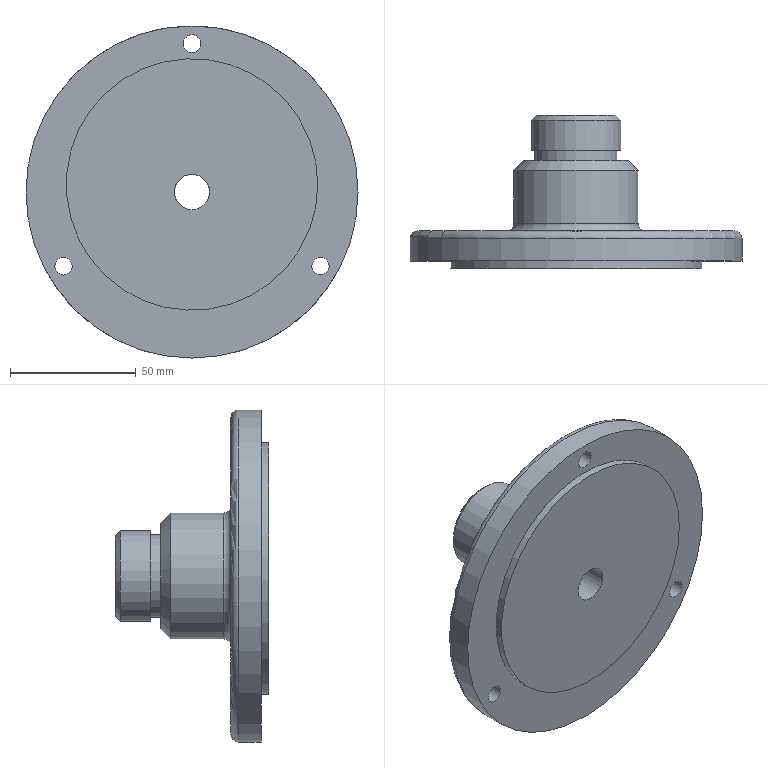Part | NX | features DATUM_CSYS 7, SKETCH 6, CBORE_HOLE 3, EXTRACT_FACE 3, EXTRUDE 3, HOLE PACKAGE 3, CHAMFER 2, Instance Feature 2, BLEND 1, Pattern Feature 1, SWP104 1 | 1 solid | 27 faces | box 132 x 61 x 132 mm | volume 237837 mm3 | cylinder 13 | plane 9 | cone 3 | torus 2 | commonest cylinder face diameters 7 x3 11 x3 14 x1 25 x1 33 x1 36 x1
STEP:
#1=CARTESIAN_POINT('',(50.,0.,3.));
#2=VERTEX_POINT('',#1);
#3=CARTESIAN_POINT('',(0.,0.,3.));
#4=DIRECTION('',(0.,-1.,0.));
#5=DIRECTION('',(1.,0.,0.));
#6=AXIS2_PLACEMENT_3D('',#3,#4,#5);
#7=CIRCLE('',#6,50.);
#8=EDGE_CURVE('',#2,#2,#7,.T.);
#9=ORIENTED_EDGE('',*,*,#8,.T.);
#10=EDGE_LOOP('',(#9));
#11=FACE_BOUND('',#10,.T.);
#12=CARTESIAN_POINT('',(50.,-3.,3.));
#13=VERTEX_POINT('',#12);
#14=CARTESIAN_POINT('',(0.,-3.,3.));
#15=DIRECTION('',(0.,-1.,0.));
#16=DIRECTION('',(1.,0.,0.));
#17=AXIS2_PLACEMENT_3D('',#14,#15,#16);
#18=CIRCLE('',#17,50.);
#19=EDGE_CURVE('',#13,#13,#18,.T.);
#20=ORIENTED_EDGE('',*,*,#19,.F.);
#21=EDGE_LOOP('',(#20));
#22=FACE_BOUND('',#21,.T.);
#23=CARTESIAN_POINT('',(0.,-3.,3.));
#24=DIRECTION('',(0.,1.,0.));
#25=DIRECTION('',(0.,0.,1.));
#26=AXIS2_PLACEMENT_3D('',#23,#24,#25);
#27=CYLINDRICAL_SURFACE('',#26,50.);
#28=ADVANCED_FACE('',(#11,#22),#27,.T.);
#29=CARTESIAN_POINT('',(7.,-3.,0.));
#30=VERTEX_POINT('',#29);
#31=CARTESIAN_POINT('',(0.,-3.,0.));
#32=DIRECTION('',(0.,-1.,0.));
#33=DIRECTION('',(1.,0.,0.));
#34=AXIS2_PLACEMENT_3D('',#31,#32,#33);
#35=CIRCLE('',#34,7.);
#36=EDGE_CURVE('',#30,#30,#35,.T.);
#37=ORIENTED_EDGE('',*,*,#36,.F.);
#38=EDGE_LOOP('',(#37));
#39=FACE_BOUND('',#38,.T.);
#40=ORIENTED_EDGE('',*,*,#19,.T.);
#41=EDGE_LOOP('',(#40));
#42=FACE_BOUND('',#41,.T.);
#43=CARTESIAN_POINT('',(0.,-3.,3.));
#44=DIRECTION('',(0.,-1.,0.));
#45=DIRECTION('',(0.,0.,-1.));
#46=AXIS2_PLACEMENT_3D('',#43,#44,#45);
#47=PLANE('',#46);
#48=ADVANCED_FACE('',(#39,#42),#47,.T.);
#49=CARTESIAN_POINT('',(0.,9.,-66.));
#50=VERTEX_POINT('',#49);
#51=CARTESIAN_POINT('',(0.,9.,0.));
#52=DIRECTION('',(0.,-1.,0.));
#53=DIRECTION('',(0.,0.,-1.));
#54=AXIS2_PLACEMENT_3D('',#51,#52,#53);
#55=CIRCLE('',#54,66.);
#56=EDGE_CURVE('',#50,#50,#55,.T.);
#57=ORIENTED_EDGE('',*,*,#56,.T.);
#58=EDGE_LOOP('',(#57));
#59=FACE_BOUND('',#58,.T.);
#60=CARTESIAN_POINT('',(66.,0.,0.));
#61=VERTEX_POINT('',#60);
#62=CARTESIAN_POINT('',(0.,0.,0.));
#63=DIRECTION('',(0.,-1.,0.));
#64=DIRECTION('',(1.,0.,0.));
#65=AXIS2_PLACEMENT_3D('',#62,#63,#64);
#66=CIRCLE('',#65,66.);
#67=EDGE_CURVE('',#61,#61,#66,.T.);
#68=ORIENTED_EDGE('',*,*,#67,.F.);
#69=EDGE_LOOP('',(#68));
#70=FACE_BOUND('',#69,.T.);
#71=CARTESIAN_POINT('',(0.,12.,0.));
#72=DIRECTION('',(0.,-1.,0.));
#73=DIRECTION('',(0.,0.,-1.));
#74=AXIS2_PLACEMENT_3D('',#71,#72,#73);
#75=CYLINDRICAL_SURFACE('',#74,66.);
#76=ADVANCED_FACE('',(#59,#70),#75,.T.);
#77=CARTESIAN_POINT('',(-51.095,0.,-33.));
#78=VERTEX_POINT('',#77);
#79=CARTESIAN_POINT('',(-51.095,0.,-29.5));
#80=DIRECTION('',(0.,-1.,0.));
#81=DIRECTION('',(0.,0.,-1.));
#82=AXIS2_PLACEMENT_3D('',#79,#80,#81);
#83=CIRCLE('',#82,3.5);
#84=EDGE_CURVE('',#78,#78,#83,.T.);
#85=ORIENTED_EDGE('',*,*,#84,.F.);
#86=EDGE_LOOP('',(#85));
#87=FACE_BOUND('',#86,.T.);
#88=CARTESIAN_POINT('',(51.095,0.,-33.));
#89=VERTEX_POINT('',#88);
#90=CARTESIAN_POINT('',(51.095,0.,-29.5));
#91=DIRECTION('',(0.,-1.,0.));
#92=DIRECTION('',(0.,0.,-1.));
#93=AXIS2_PLACEMENT_3D('',#90,#91,#92);
#94=CIRCLE('',#93,3.5);
#95=EDGE_CURVE('',#89,#89,#94,.T.);
#96=ORIENTED_EDGE('',*,*,#95,.F.);
#97=EDGE_LOOP('',(#96));
#98=FACE_BOUND('',#97,.T.);
#99=CARTESIAN_POINT('',(0.,0.,55.5));
#100=VERTEX_POINT('',#99);
#101=CARTESIAN_POINT('',(0.,0.,59.));
#102=DIRECTION('',(0.,-1.,0.));
#103=DIRECTION('',(0.,0.,-1.));
#104=AXIS2_PLACEMENT_3D('',#101,#102,#103);
#105=CIRCLE('',#104,3.5);
#106=EDGE_CURVE('',#100,#100,#105,.T.);
#107=ORIENTED_EDGE('',*,*,#106,.F.);
#108=EDGE_LOOP('',(#107));
#109=FACE_BOUND('',#108,.T.);
#110=ORIENTED_EDGE('',*,*,#67,.T.);
#111=EDGE_LOOP('',(#110));
#112=FACE_BOUND('',#111,.T.);
#113=ORIENTED_EDGE('',*,*,#8,.F.);
#114=EDGE_LOOP('',(#113));
#115=FACE_BOUND('',#114,.T.);
#116=CARTESIAN_POINT('',(0.,0.,1.5));
#117=DIRECTION('',(0.,-1.,0.));
#118=DIRECTION('',(0.,0.,-1.));
#119=AXIS2_PLACEMENT_3D('',#116,#117,#118);
#120=PLANE('',#119);
#121=ADVANCED_FACE('',(#87,#98,#109,#112,#115),#120,.T.);
#122=CARTESIAN_POINT('',(52.506,12.,-34.816));
#123=VERTEX_POINT('',#122);
#124=CARTESIAN_POINT('',(-52.506,12.,-34.816));
#125=VERTEX_POINT('',#124);
#126=CARTESIAN_POINT('',(0.,12.,0.));
#127=DIRECTION('',(0.,-1.,0.));
#128=DIRECTION('',(0.,0.,-1.));
#129=AXIS2_PLACEMENT_3D('',#126,#127,#128);
#130=CIRCLE('',#129,63.);
#131=EDGE_CURVE('',#123,#125,#130,.F.);
#132=ORIENTED_EDGE('',*,*,#131,.T.);
#133=CARTESIAN_POINT('',(-56.404,12.,-28.063));
#134=VERTEX_POINT('',#133);
#135=CARTESIAN_POINT('',(-51.095,12.,-29.5));
#136=DIRECTION('',(0.,-1.,0.));
#137=DIRECTION('',(0.,0.,-1.));
#138=AXIS2_PLACEMENT_3D('',#135,#136,#137);
#139=CIRCLE('',#138,5.5);
#140=EDGE_CURVE('',#125,#134,#139,.T.);
#141=ORIENTED_EDGE('',*,*,#140,.T.);
#142=CARTESIAN_POINT('',(-3.899,12.,62.879));
#143=VERTEX_POINT('',#142);
#144=CARTESIAN_POINT('',(0.,12.,0.));
#145=DIRECTION('',(0.,-1.,0.));
#146=DIRECTION('',(0.,0.,-1.));
#147=AXIS2_PLACEMENT_3D('',#144,#145,#146);
#148=CIRCLE('',#147,63.);
#149=EDGE_CURVE('',#134,#143,#148,.F.);
#150=ORIENTED_EDGE('',*,*,#149,.T.);
#151=CARTESIAN_POINT('',(3.899,12.,62.879));
#152=VERTEX_POINT('',#151);
#153=CARTESIAN_POINT('',(0.,12.,59.));
#154=DIRECTION('',(0.,-1.,0.));
#155=DIRECTION('',(0.,0.,-1.));
#156=AXIS2_PLACEMENT_3D('',#153,#154,#155);
#157=CIRCLE('',#156,5.5);
#158=EDGE_CURVE('',#143,#152,#157,.T.);
#159=ORIENTED_EDGE('',*,*,#158,.T.);
#160=CARTESIAN_POINT('',(56.404,12.,-28.063));
#161=VERTEX_POINT('',#160);
#162=CARTESIAN_POINT('',(0.,12.,0.));
#163=DIRECTION('',(0.,-1.,0.));
#164=DIRECTION('',(0.,0.,-1.));
#165=AXIS2_PLACEMENT_3D('',#162,#163,#164);
#166=CIRCLE('',#165,63.);
#167=EDGE_CURVE('',#152,#161,#166,.F.);
#168=ORIENTED_EDGE('',*,*,#167,.T.);
#169=CARTESIAN_POINT('',(51.095,12.,-29.5));
#170=DIRECTION('',(0.,-1.,0.));
#171=DIRECTION('',(0.,0.,-1.));
#172=AXIS2_PLACEMENT_3D('',#169,#170,#171);
#173=CIRCLE('',#172,5.5);
#174=EDGE_CURVE('',#161,#123,#173,.T.);
#175=ORIENTED_EDGE('',*,*,#174,.T.);
#176=EDGE_LOOP('',(#132,#141,#150,#159,#168,#175));
#177=FACE_BOUND('',#176,.T.);
#178=CARTESIAN_POINT('',(0.,12.,-28.));
#179=VERTEX_POINT('',#178);
#180=CARTESIAN_POINT('',(0.,12.,0.));
#181=DIRECTION('',(0.,-1.,0.));
#182=DIRECTION('',(0.,0.,-1.));
#183=AXIS2_PLACEMENT_3D('',#180,#181,#182);
#184=CIRCLE('',#183,28.);
#185=EDGE_CURVE('',#179,#179,#184,.T.);
#186=ORIENTED_EDGE('',*,*,#185,.T.);
#187=EDGE_LOOP('',(#186));
#188=FACE_BOUND('',#187,.T.);
#189=CARTESIAN_POINT('',(0.,12.,3.));
#190=DIRECTION('',(0.,-1.,0.));
#191=DIRECTION('',(0.,0.,-1.));
#192=AXIS2_PLACEMENT_3D('',#189,#190,#191);
#193=PLANE('',#192);
#194=ADVANCED_FACE('',(#177,#188),#193,.F.);
#195=CARTESIAN_POINT('',(0.,29.825,-7.));
#196=VERTEX_POINT('',#195);
#197=CARTESIAN_POINT('',(0.,29.825,0.));
#198=DIRECTION('',(0.,-1.,0.));
#199=DIRECTION('',(0.,0.,-1.));
#200=AXIS2_PLACEMENT_3D('',#197,#198,#199);
#201=CIRCLE('',#200,7.);
#202=EDGE_CURVE('',#196,#196,#201,.T.);
#203=ORIENTED_EDGE('',*,*,#202,.F.);
#204=EDGE_LOOP('',(#203));
#205=FACE_BOUND('',#204,.T.);
#206=ORIENTED_EDGE('',*,*,#36,.T.);
#207=EDGE_LOOP('',(#206));
#208=FACE_BOUND('',#207,.T.);
#209=CARTESIAN_POINT('',(0.,58.,0.));
#210=DIRECTION('',(0.,-1.,0.));
#211=DIRECTION('',(0.,0.,-1.));
#212=AXIS2_PLACEMENT_3D('',#209,#210,#211);
#213=CYLINDRICAL_SURFACE('',#212,7.);
#214=ADVANCED_FACE('',(#205,#208),#213,.F.);
#215=CARTESIAN_POINT('',(0.,33.,-12.5));
#216=VERTEX_POINT('',#215);
#217=CARTESIAN_POINT('',(0.,33.,0.));
#218=DIRECTION('',(0.,-1.,0.));
#219=DIRECTION('',(0.,0.,-1.));
#220=AXIS2_PLACEMENT_3D('',#217,#218,#219);
#221=CIRCLE('',#220,12.5);
#222=EDGE_CURVE('',#216,#216,#221,.T.);
#223=ORIENTED_EDGE('',*,*,#222,.F.);
#224=EDGE_LOOP('',(#223));
#225=FACE_BOUND('',#224,.T.);
#226=ORIENTED_EDGE('',*,*,#202,.T.);
#227=EDGE_LOOP('',(#226));
#228=FACE_BOUND('',#227,.T.);
#229=CARTESIAN_POINT('',(0.,29.825,0.));
#230=DIRECTION('',(0.,1.,0.));
#231=DIRECTION('',(0.,0.,1.));
#232=AXIS2_PLACEMENT_3D('',#229,#230,#231);
#233=CONICAL_SURFACE('',#232,7.,1.047);
#234=ADVANCED_FACE('',(#225,#228),#233,.F.);
#235=CARTESIAN_POINT('',(0.,58.,-12.5));
#236=VERTEX_POINT('',#235);
#237=CARTESIAN_POINT('',(0.,58.,0.));
#238=DIRECTION('',(0.,-1.,0.));
#239=DIRECTION('',(0.,0.,-1.));
#240=AXIS2_PLACEMENT_3D('',#237,#238,#239);
#241=CIRCLE('',#240,12.5);
#242=EDGE_CURVE('',#236,#236,#241,.T.);
#243=ORIENTED_EDGE('',*,*,#242,.F.);
#244=EDGE_LOOP('',(#243));
#245=FACE_BOUND('',#244,.T.);
#246=ORIENTED_EDGE('',*,*,#222,.T.);
#247=EDGE_LOOP('',(#246));
#248=FACE_BOUND('',#247,.T.);
#249=CARTESIAN_POINT('',(0.,58.,0.));
#250=DIRECTION('',(0.,-1.,0.));
#251=DIRECTION('',(0.,0.,-1.));
#252=AXIS2_PLACEMENT_3D('',#249,#250,#251);
#253=CYLINDRICAL_SURFACE('',#252,12.5);
#254=ADVANCED_FACE('',(#245,#248),#253,.F.);
#255=CARTESIAN_POINT('',(0.,58.,-16.));
#256=VERTEX_POINT('',#255);
#257=CARTESIAN_POINT('',(0.,58.,0.));
#258=DIRECTION('',(0.,-1.,0.));
#259=DIRECTION('',(0.,0.,-1.));
#260=AXIS2_PLACEMENT_3D('',#257,#258,#259);
#261=CIRCLE('',#260,16.);
#262=EDGE_CURVE('',#256,#256,#261,.F.);
#263=ORIENTED_EDGE('',*,*,#262,.T.);
#264=EDGE_LOOP('',(#263));
#265=FACE_BOUND('',#264,.T.);
#266=ORIENTED_EDGE('',*,*,#242,.T.);
#267=EDGE_LOOP('',(#266));
#268=FACE_BOUND('',#267,.T.);
#269=CARTESIAN_POINT('',(0.,58.,12.5));
#270=DIRECTION('',(0.,-1.,0.));
#271=DIRECTION('',(0.,0.,-1.));
#272=AXIS2_PLACEMENT_3D('',#269,#270,#271);
#273=PLANE('',#272);
#274=ADVANCED_FACE('',(#265,#268),#273,.F.);
#275=CARTESIAN_POINT('',(0.,56.,-18.));
#276=VERTEX_POINT('',#275);
#277=CARTESIAN_POINT('',(0.,56.,0.));
#278=DIRECTION('',(0.,-1.,0.));
#279=DIRECTION('',(0.,0.,-1.));
#280=AXIS2_PLACEMENT_3D('',#277,#278,#279);
#281=CIRCLE('',#280,18.);
#282=EDGE_CURVE('',#276,#276,#281,.T.);
#283=ORIENTED_EDGE('',*,*,#282,.T.);
#284=EDGE_LOOP('',(#283));
#285=FACE_BOUND('',#284,.T.);
#286=CARTESIAN_POINT('',(0.,44.,-18.));
#287=VERTEX_POINT('',#286);
#288=CARTESIAN_POINT('',(0.,44.,0.));
#289=DIRECTION('',(0.,-1.,0.));
#290=DIRECTION('',(0.,0.,-1.));
#291=AXIS2_PLACEMENT_3D('',#288,#289,#290);
#292=CIRCLE('',#291,18.);
#293=EDGE_CURVE('',#287,#287,#292,.T.);
#294=ORIENTED_EDGE('',*,*,#293,.F.);
#295=EDGE_LOOP('',(#294));
#296=FACE_BOUND('',#295,.T.);
#297=CARTESIAN_POINT('',(0.,58.,0.));
#298=DIRECTION('',(0.,-1.,0.));
#299=DIRECTION('',(0.,0.,-1.));
#300=AXIS2_PLACEMENT_3D('',#297,#298,#299);
#301=CYLINDRICAL_SURFACE('',#300,18.);
#302=ADVANCED_FACE('',(#285,#296),#301,.T.);
#303=CARTESIAN_POINT('',(0.,44.,-16.5));
#304=VERTEX_POINT('',#303);
#305=CARTESIAN_POINT('',(0.,44.,0.));
#306=DIRECTION('',(0.,-1.,0.));
#307=DIRECTION('',(0.,0.,-1.));
#308=AXIS2_PLACEMENT_3D('',#305,#306,#307);
#309=CIRCLE('',#308,16.5);
#310=EDGE_CURVE('',#304,#304,#309,.T.);
#311=ORIENTED_EDGE('',*,*,#310,.F.);
#312=EDGE_LOOP('',(#311));
#313=FACE_BOUND('',#312,.T.);
#314=ORIENTED_EDGE('',*,*,#293,.T.);
#315=EDGE_LOOP('',(#314));
#316=FACE_BOUND('',#315,.T.);
#317=CARTESIAN_POINT('',(0.,44.,18.));
#318=DIRECTION('',(0.,1.,0.));
#319=DIRECTION('',(0.,0.,1.));
#320=AXIS2_PLACEMENT_3D('',#317,#318,#319);
#321=PLANE('',#320);
#322=ADVANCED_FACE('',(#313,#316),#321,.F.);
#323=CARTESIAN_POINT('',(0.,40.,-16.5));
#324=VERTEX_POINT('',#323);
#325=CARTESIAN_POINT('',(0.,40.,0.));
#326=DIRECTION('',(0.,-1.,0.));
#327=DIRECTION('',(0.,0.,-1.));
#328=AXIS2_PLACEMENT_3D('',#325,#326,#327);
#329=CIRCLE('',#328,16.5);
#330=EDGE_CURVE('',#324,#324,#329,.T.);
#331=ORIENTED_EDGE('',*,*,#330,.F.);
#332=EDGE_LOOP('',(#331));
#333=FACE_BOUND('',#332,.T.);
#334=ORIENTED_EDGE('',*,*,#310,.T.);
#335=EDGE_LOOP('',(#334));
#336=FACE_BOUND('',#335,.T.);
#337=CARTESIAN_POINT('',(0.,58.,0.));
#338=DIRECTION('',(0.,-1.,0.));
#339=DIRECTION('',(0.,0.,-1.));
#340=AXIS2_PLACEMENT_3D('',#337,#338,#339);
#341=CYLINDRICAL_SURFACE('',#340,16.5);
#342=ADVANCED_FACE('',(#333,#336),#341,.T.);
#343=CARTESIAN_POINT('',(0.,40.,-21.));
#344=VERTEX_POINT('',#343);
#345=CARTESIAN_POINT('',(0.,40.,0.));
#346=DIRECTION('',(0.,-1.,0.));
#347=DIRECTION('',(0.,0.,-1.));
#348=AXIS2_PLACEMENT_3D('',#345,#346,#347);
#349=CIRCLE('',#348,21.);
#350=EDGE_CURVE('',#344,#344,#349,.F.);
#351=ORIENTED_EDGE('',*,*,#350,.T.);
#352=EDGE_LOOP('',(#351));
#353=FACE_BOUND('',#352,.T.);
#354=ORIENTED_EDGE('',*,*,#330,.T.);
#355=EDGE_LOOP('',(#354));
#356=FACE_BOUND('',#355,.T.);
#357=CARTESIAN_POINT('',(0.,40.,16.5));
#358=DIRECTION('',(0.,-1.,0.));
#359=DIRECTION('',(0.,0.,-1.));
#360=AXIS2_PLACEMENT_3D('',#357,#358,#359);
#361=PLANE('',#360);
#362=ADVANCED_FACE('',(#353,#356),#361,.F.);
#363=CARTESIAN_POINT('',(0.,15.,-25.));
#364=VERTEX_POINT('',#363);
#365=CARTESIAN_POINT('',(0.,15.,0.));
#366=DIRECTION('',(0.,-1.,0.));
#367=DIRECTION('',(0.,0.,-1.));
#368=AXIS2_PLACEMENT_3D('',#365,#366,#367);
#369=CIRCLE('',#368,25.);
#370=EDGE_CURVE('',#364,#364,#369,.F.);
#371=ORIENTED_EDGE('',*,*,#370,.T.);
#372=EDGE_LOOP('',(#371));
#373=FACE_BOUND('',#372,.T.);
#374=CARTESIAN_POINT('',(0.,36.,-25.));
#375=VERTEX_POINT('',#374);
#376=CARTESIAN_POINT('',(0.,36.,0.));
#377=DIRECTION('',(0.,-1.,0.));
#378=DIRECTION('',(0.,0.,-1.));
#379=AXIS2_PLACEMENT_3D('',#376,#377,#378);
#380=CIRCLE('',#379,25.);
#381=EDGE_CURVE('',#375,#375,#380,.T.);
#382=ORIENTED_EDGE('',*,*,#381,.T.);
#383=EDGE_LOOP('',(#382));
#384=FACE_BOUND('',#383,.T.);
#385=CARTESIAN_POINT('',(0.,58.,0.));
#386=DIRECTION('',(0.,-1.,0.));
#387=DIRECTION('',(0.,0.,-1.));
#388=AXIS2_PLACEMENT_3D('',#385,#386,#387);
#389=CYLINDRICAL_SURFACE('',#388,25.);
#390=ADVANCED_FACE('',(#373,#384),#389,.T.);
#391=ORIENTED_EDGE('',*,*,#350,.F.);
#392=EDGE_LOOP('',(#391));
#393=FACE_BOUND('',#392,.T.);
#394=ORIENTED_EDGE('',*,*,#381,.F.);
#395=EDGE_LOOP('',(#394));
#396=FACE_BOUND('',#395,.T.);
#397=CARTESIAN_POINT('',(0.,36.,0.));
#398=DIRECTION('',(0.,-1.,0.));
#399=DIRECTION('',(0.,0.,-1.));
#400=AXIS2_PLACEMENT_3D('',#397,#398,#399);
#401=CONICAL_SURFACE('',#400,25.,0.7854);
#402=ADVANCED_FACE('',(#393,#396),#401,.T.);
#403=ORIENTED_EDGE('',*,*,#262,.F.);
#404=EDGE_LOOP('',(#403));
#405=FACE_BOUND('',#404,.T.);
#406=ORIENTED_EDGE('',*,*,#282,.F.);
#407=EDGE_LOOP('',(#406));
#408=FACE_BOUND('',#407,.T.);
#409=CARTESIAN_POINT('',(0.,56.,0.));
#410=DIRECTION('',(0.,-1.,0.));
#411=DIRECTION('',(0.,0.,-1.));
#412=AXIS2_PLACEMENT_3D('',#409,#410,#411);
#413=CONICAL_SURFACE('',#412,18.,0.7854);
#414=ADVANCED_FACE('',(#405,#408),#413,.T.);
#415=CARTESIAN_POINT('',(-52.506,12.,-34.816));
#416=CARTESIAN_POINT('',(-53.909,12.,-34.444));
#417=CARTESIAN_POINT('',(-56.368,11.196,-32.553));
#418=CARTESIAN_POINT('',(-56.783,12.,-29.462));
#419=CARTESIAN_POINT('',(-56.404,12.,-28.063));
#420=B_SPLINE_CURVE_WITH_KNOTS('',3,(#415,#416,#417,#418,#419),.UNSPECIFIED.,.F.,.F.,(4,1,4),(0.005193,0.009546,0.0139),.UNSPECIFIED.);
#421=EDGE_CURVE('',#125,#134,#420,.T.);
#422=ORIENTED_EDGE('',*,*,#421,.F.);
#423=ORIENTED_EDGE('',*,*,#131,.F.);
#424=CARTESIAN_POINT('',(56.404,12.,-28.063));
#425=CARTESIAN_POINT('',(56.784,12.,-29.465));
#426=CARTESIAN_POINT('',(56.376,11.196,-32.539));
#427=CARTESIAN_POINT('',(53.906,12.,-34.445));
#428=CARTESIAN_POINT('',(52.506,12.,-34.816));
#429=B_SPLINE_CURVE_WITH_KNOTS('',3,(#424,#425,#426,#427,#428),.UNSPECIFIED.,.F.,.F.,(4,1,4),(0.005193,0.009546,0.0139),.UNSPECIFIED.);
#430=EDGE_CURVE('',#161,#123,#429,.T.);
#431=ORIENTED_EDGE('',*,*,#430,.F.);
#432=ORIENTED_EDGE('',*,*,#167,.F.);
#433=CARTESIAN_POINT('',(-3.899,12.,62.879));
#434=CARTESIAN_POINT('',(-2.875,12.,63.909));
#435=CARTESIAN_POINT('',(-0.008151,11.196,65.092));
#436=CARTESIAN_POINT('',(2.877,12.,63.907));
#437=CARTESIAN_POINT('',(3.899,12.,62.879));
#438=B_SPLINE_CURVE_WITH_KNOTS('',3,(#433,#434,#435,#436,#437),.UNSPECIFIED.,.F.,.F.,(4,1,4),(0.005193,0.009546,0.0139),.UNSPECIFIED.);
#439=EDGE_CURVE('',#143,#152,#438,.T.);
#440=ORIENTED_EDGE('',*,*,#439,.F.);
#441=ORIENTED_EDGE('',*,*,#149,.F.);
#442=EDGE_LOOP('',(#422,#423,#431,#432,#440,#441));
#443=FACE_BOUND('',#442,.T.);
#444=ORIENTED_EDGE('',*,*,#56,.F.);
#445=EDGE_LOOP('',(#444));
#446=FACE_BOUND('',#445,.T.);
#447=CARTESIAN_POINT('',(0.,9.,0.));
#448=DIRECTION('',(0.,-1.,0.));
#449=DIRECTION('',(0.,0.,-1.));
#450=AXIS2_PLACEMENT_3D('',#447,#448,#449);
#451=TOROIDAL_SURFACE('',#450,63.,3.);
#452=ADVANCED_FACE('',(#443,#446),#451,.T.);
#453=ORIENTED_EDGE('',*,*,#370,.F.);
#454=EDGE_LOOP('',(#453));
#455=FACE_BOUND('',#454,.T.);
#456=ORIENTED_EDGE('',*,*,#185,.F.);
#457=EDGE_LOOP('',(#456));
#458=FACE_BOUND('',#457,.T.);
#459=CARTESIAN_POINT('',(0.,15.,0.));
#460=DIRECTION('',(0.,-1.,0.));
#461=DIRECTION('',(0.,0.,-1.));
#462=AXIS2_PLACEMENT_3D('',#459,#460,#461);
#463=TOROIDAL_SURFACE('',#462,28.,3.);
#464=ADVANCED_FACE('',(#455,#458),#463,.F.);
#465=ORIENTED_EDGE('',*,*,#106,.T.);
#466=EDGE_LOOP('',(#465));
#467=FACE_BOUND('',#466,.T.);
#468=CARTESIAN_POINT('',(0.,6.,55.5));
#469=VERTEX_POINT('',#468);
#470=CARTESIAN_POINT('',(0.,6.,59.));
#471=DIRECTION('',(0.,-1.,0.));
#472=DIRECTION('',(0.,0.,-1.));
#473=AXIS2_PLACEMENT_3D('',#470,#471,#472);
#474=CIRCLE('',#473,3.5);
#475=EDGE_CURVE('',#469,#469,#474,.F.);
#476=ORIENTED_EDGE('',*,*,#475,.T.);
#477=EDGE_LOOP('',(#476));
#478=FACE_BOUND('',#477,.T.);
#479=CARTESIAN_POINT('',(0.,-62.977,59.));
#480=DIRECTION('',(0.,-1.,0.));
#481=DIRECTION('',(0.,0.,-1.));
#482=AXIS2_PLACEMENT_3D('',#479,#480,#481);
#483=CYLINDRICAL_SURFACE('',#482,3.5);
#484=ADVANCED_FACE('',(#467,#478),#483,.F.);
#485=ORIENTED_EDGE('',*,*,#475,.F.);
#486=EDGE_LOOP('',(#485));
#487=FACE_BOUND('',#486,.T.);
#488=CARTESIAN_POINT('',(0.,6.,53.5));
#489=VERTEX_POINT('',#488);
#490=CARTESIAN_POINT('',(0.,6.,59.));
#491=DIRECTION('',(0.,-1.,0.));
#492=DIRECTION('',(0.,0.,-1.));
#493=AXIS2_PLACEMENT_3D('',#490,#491,#492);
#494=CIRCLE('',#493,5.5);
#495=EDGE_CURVE('',#489,#489,#494,.F.);
#496=ORIENTED_EDGE('',*,*,#495,.T.);
#497=EDGE_LOOP('',(#496));
#498=FACE_BOUND('',#497,.T.);
#499=CARTESIAN_POINT('',(0.,6.,59.));
#500=DIRECTION('',(0.,-1.,0.));
#501=DIRECTION('',(0.,0.,-1.));
#502=AXIS2_PLACEMENT_3D('',#499,#500,#501);
#503=PLANE('',#502);
#504=ADVANCED_FACE('',(#487,#498),#503,.F.);
#505=ORIENTED_EDGE('',*,*,#439,.T.);
#506=ORIENTED_EDGE('',*,*,#158,.F.);
#507=EDGE_LOOP('',(#505,#506));
#508=FACE_BOUND('',#507,.T.);
#509=ORIENTED_EDGE('',*,*,#495,.F.);
#510=EDGE_LOOP('',(#509));
#511=FACE_BOUND('',#510,.T.);
#512=CARTESIAN_POINT('',(0.,12.,59.));
#513=DIRECTION('',(0.,-1.,0.));
#514=DIRECTION('',(0.,0.,-1.));
#515=AXIS2_PLACEMENT_3D('',#512,#513,#514);
#516=CYLINDRICAL_SURFACE('',#515,5.5);
#517=ADVANCED_FACE('',(#508,#511),#516,.F.);
#518=ORIENTED_EDGE('',*,*,#95,.T.);
#519=EDGE_LOOP('',(#518));
#520=FACE_BOUND('',#519,.T.);
#521=CARTESIAN_POINT('',(51.095,6.,-33.));
#522=VERTEX_POINT('',#521);
#523=CARTESIAN_POINT('',(51.095,6.,-29.5));
#524=DIRECTION('',(0.,-1.,0.));
#525=DIRECTION('',(0.,0.,-1.));
#526=AXIS2_PLACEMENT_3D('',#523,#524,#525);
#527=CIRCLE('',#526,3.5);
#528=EDGE_CURVE('',#522,#522,#527,.F.);
#529=ORIENTED_EDGE('',*,*,#528,.T.);
#530=EDGE_LOOP('',(#529));
#531=FACE_BOUND('',#530,.T.);
#532=CARTESIAN_POINT('',(51.095,-62.977,-29.5));
#533=DIRECTION('',(0.,-1.,0.));
#534=DIRECTION('',(0.,0.,-1.));
#535=AXIS2_PLACEMENT_3D('',#532,#533,#534);
#536=CYLINDRICAL_SURFACE('',#535,3.5);
#537=ADVANCED_FACE('',(#520,#531),#536,.F.);
#538=ORIENTED_EDGE('',*,*,#528,.F.);
#539=EDGE_LOOP('',(#538));
#540=FACE_BOUND('',#539,.T.);
#541=CARTESIAN_POINT('',(51.095,6.,-35.));
#542=VERTEX_POINT('',#541);
#543=CARTESIAN_POINT('',(51.095,6.,-29.5));
#544=DIRECTION('',(0.,-1.,0.));
#545=DIRECTION('',(0.,0.,-1.));
#546=AXIS2_PLACEMENT_3D('',#543,#544,#545);
#547=CIRCLE('',#546,5.5);
#548=EDGE_CURVE('',#542,#542,#547,.F.);
#549=ORIENTED_EDGE('',*,*,#548,.T.);
#550=EDGE_LOOP('',(#549));
#551=FACE_BOUND('',#550,.T.);
#552=CARTESIAN_POINT('',(51.095,6.,-29.5));
#553=DIRECTION('',(0.,-1.,0.));
#554=DIRECTION('',(0.,0.,-1.));
#555=AXIS2_PLACEMENT_3D('',#552,#553,#554);
#556=PLANE('',#555);
#557=ADVANCED_FACE('',(#540,#551),#556,.F.);
#558=ORIENTED_EDGE('',*,*,#430,.T.);
#559=ORIENTED_EDGE('',*,*,#174,.F.);
#560=EDGE_LOOP('',(#558,#559));
#561=FACE_BOUND('',#560,.T.);
#562=ORIENTED_EDGE('',*,*,#548,.F.);
#563=EDGE_LOOP('',(#562));
#564=FACE_BOUND('',#563,.T.);
#565=CARTESIAN_POINT('',(51.095,12.,-29.5));
#566=DIRECTION('',(0.,-1.,0.));
#567=DIRECTION('',(0.,0.,-1.));
#568=AXIS2_PLACEMENT_3D('',#565,#566,#567);
#569=CYLINDRICAL_SURFACE('',#568,5.5);
#570=ADVANCED_FACE('',(#561,#564),#569,.F.);
#571=ORIENTED_EDGE('',*,*,#84,.T.);
#572=EDGE_LOOP('',(#571));
#573=FACE_BOUND('',#572,.T.);
#574=CARTESIAN_POINT('',(-51.095,6.,-33.));
#575=VERTEX_POINT('',#574);
#576=CARTESIAN_POINT('',(-51.095,6.,-29.5));
#577=DIRECTION('',(0.,-1.,0.));
#578=DIRECTION('',(0.,0.,-1.));
#579=AXIS2_PLACEMENT_3D('',#576,#577,#578);
#580=CIRCLE('',#579,3.5);
#581=EDGE_CURVE('',#575,#575,#580,.F.);
#582=ORIENTED_EDGE('',*,*,#581,.T.);
#583=EDGE_LOOP('',(#582));
#584=FACE_BOUND('',#583,.T.);
#585=CARTESIAN_POINT('',(-51.095,-62.977,-29.5));
#586=DIRECTION('',(0.,-1.,0.));
#587=DIRECTION('',(0.,0.,-1.));
#588=AXIS2_PLACEMENT_3D('',#585,#586,#587);
#589=CYLINDRICAL_SURFACE('',#588,3.5);
#590=ADVANCED_FACE('',(#573,#584),#589,.F.);
#591=ORIENTED_EDGE('',*,*,#581,.F.);
#592=EDGE_LOOP('',(#591));
#593=FACE_BOUND('',#592,.T.);
#594=CARTESIAN_POINT('',(-51.095,6.,-35.));
#595=VERTEX_POINT('',#594);
#596=CARTESIAN_POINT('',(-51.095,6.,-29.5));
#597=DIRECTION('',(0.,-1.,0.));
#598=DIRECTION('',(0.,0.,-1.));
#599=AXIS2_PLACEMENT_3D('',#596,#597,#598);
#600=CIRCLE('',#599,5.5);
#601=EDGE_CURVE('',#595,#595,#600,.F.);
#602=ORIENTED_EDGE('',*,*,#601,.T.);
#603=EDGE_LOOP('',(#602));
#604=FACE_BOUND('',#603,.T.);
#605=CARTESIAN_POINT('',(-51.095,6.,-29.5));
#606=DIRECTION('',(0.,-1.,0.));
#607=DIRECTION('',(0.,0.,-1.));
#608=AXIS2_PLACEMENT_3D('',#605,#606,#607);
#609=PLANE('',#608);
#610=ADVANCED_FACE('',(#593,#604),#609,.F.);
#611=ORIENTED_EDGE('',*,*,#421,.T.);
#612=ORIENTED_EDGE('',*,*,#140,.F.);
#613=EDGE_LOOP('',(#611,#612));
#614=FACE_BOUND('',#613,.T.);
#615=ORIENTED_EDGE('',*,*,#601,.F.);
#616=EDGE_LOOP('',(#615));
#617=FACE_BOUND('',#616,.T.);
#618=CARTESIAN_POINT('',(-51.095,12.,-29.5));
#619=DIRECTION('',(0.,-1.,0.));
#620=DIRECTION('',(0.,0.,-1.));
#621=AXIS2_PLACEMENT_3D('',#618,#619,#620);
#622=CYLINDRICAL_SURFACE('',#621,5.5);
#623=ADVANCED_FACE('',(#614,#617),#622,.F.);
#624=CLOSED_SHELL('',(#28,#48,#76,#121,#194,#214,#234,#254,#274,#302,#322,#342,#362,#390,#402,#414,#452,#464,#484,#504,#517,#537,#557,#570,#590,#610,#623));
#625=MANIFOLD_SOLID_BREP('',#624);
#626=(LENGTH_UNIT()NAMED_UNIT(*)SI_UNIT(.MILLI.,.METRE.));
#627=UNCERTAINTY_MEASURE_WITH_UNIT(LENGTH_MEASURE(0.0508),#626,'','');
#628=(NAMED_UNIT(*)PLANE_ANGLE_UNIT()SI_UNIT($,.RADIAN.));
#629=(NAMED_UNIT(*)SI_UNIT($,.STERADIAN.)SOLID_ANGLE_UNIT());
#630=(GEOMETRIC_REPRESENTATION_CONTEXT(3)GLOBAL_UNCERTAINTY_ASSIGNED_CONTEXT((#627))GLOBAL_UNIT_ASSIGNED_CONTEXT((#626,#628,#629))REPRESENTATION_CONTEXT('',''));
#631=ADVANCED_BREP_SHAPE_REPRESENTATION('',(#625),#630);